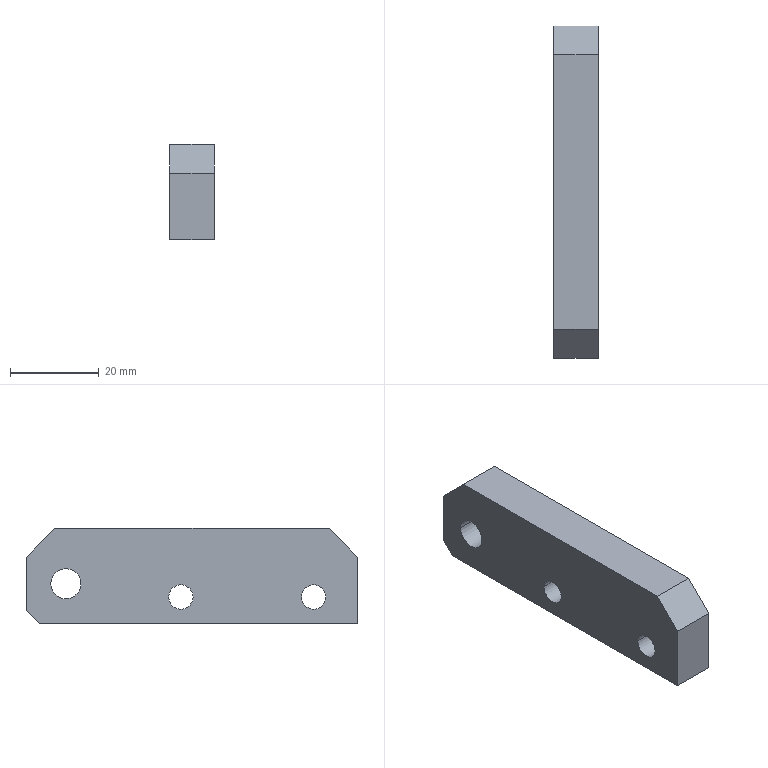Part | NX | features 001 2 | 1 solid | 15 faces | box 10 x 75 x 21.5 mm | volume 14819 mm3 | plane 9 | cylinder 6 | commonest cylinder face diameters 5.5 x4 6.8 x2
STEP:
#1=CARTESIAN_POINT('',(-195.,37.25,-6.));
#2=VERTEX_POINT('',#1);
#3=CARTESIAN_POINT('',(-205.,37.25,-6.));
#4=VERTEX_POINT('',#3);
#5=CARTESIAN_POINT('',(-195.,37.25,-6.));
#6=DIRECTION('',(-1.,0.,0.));
#7=VECTOR('',#6,1000.);
#8=LINE('',#5,#7);
#9=EDGE_CURVE('',#2,#4,#8,.T.);
#10=ORIENTED_EDGE('',*,*,#9,.F.);
#11=CARTESIAN_POINT('',(-195.,42.75,-6.));
#12=VERTEX_POINT('',#11);
#13=CARTESIAN_POINT('',(-195.,40.,-6.));
#14=DIRECTION('',(-1.,0.,0.));
#15=DIRECTION('',(0.,1.,0.));
#16=AXIS2_PLACEMENT_3D('',#13,#14,#15);
#17=CIRCLE('',#16,2.75);
#18=EDGE_CURVE('',#12,#2,#17,.T.);
#19=ORIENTED_EDGE('',*,*,#18,.F.);
#20=CARTESIAN_POINT('',(-205.,42.75,-6.));
#21=VERTEX_POINT('',#20);
#22=CARTESIAN_POINT('',(-195.,42.75,-6.));
#23=DIRECTION('',(-1.,0.,0.));
#24=VECTOR('',#23,1000.);
#25=LINE('',#22,#24);
#26=EDGE_CURVE('',#21,#12,#25,.F.);
#27=ORIENTED_EDGE('',*,*,#26,.F.);
#28=CARTESIAN_POINT('',(-205.,40.,-6.));
#29=DIRECTION('',(1.,0.,0.));
#30=DIRECTION('',(0.,-1.,0.));
#31=AXIS2_PLACEMENT_3D('',#28,#29,#30);
#32=CIRCLE('',#31,2.75);
#33=EDGE_CURVE('',#4,#21,#32,.T.);
#34=ORIENTED_EDGE('',*,*,#33,.F.);
#35=EDGE_LOOP('',(#10,#19,#27,#34));
#36=FACE_BOUND('',#35,.T.);
#37=CARTESIAN_POINT('',(-195.,40.,-6.));
#38=DIRECTION('',(1.,0.,0.));
#39=DIRECTION('',(0.,1.,0.));
#40=AXIS2_PLACEMENT_3D('',#37,#38,#39);
#41=CYLINDRICAL_SURFACE('',#40,2.75);
#42=ADVANCED_FACE('',(#36),#41,.F.);
#43=CARTESIAN_POINT('',(-205.,40.,-6.));
#44=DIRECTION('',(1.,0.,0.));
#45=DIRECTION('',(0.,1.,0.));
#46=AXIS2_PLACEMENT_3D('',#43,#44,#45);
#47=CIRCLE('',#46,2.75);
#48=EDGE_CURVE('',#21,#4,#47,.T.);
#49=ORIENTED_EDGE('',*,*,#48,.F.);
#50=ORIENTED_EDGE('',*,*,#26,.T.);
#51=CARTESIAN_POINT('',(-195.,40.,-6.));
#52=DIRECTION('',(-1.,0.,0.));
#53=DIRECTION('',(0.,-1.,0.));
#54=AXIS2_PLACEMENT_3D('',#51,#52,#53);
#55=CIRCLE('',#54,2.75);
#56=EDGE_CURVE('',#2,#12,#55,.T.);
#57=ORIENTED_EDGE('',*,*,#56,.F.);
#58=ORIENTED_EDGE('',*,*,#9,.T.);
#59=EDGE_LOOP('',(#49,#50,#57,#58));
#60=FACE_BOUND('',#59,.T.);
#61=CARTESIAN_POINT('',(-195.,40.,-6.));
#62=DIRECTION('',(1.,0.,0.));
#63=DIRECTION('',(0.,1.,0.));
#64=AXIS2_PLACEMENT_3D('',#61,#62,#63);
#65=CYLINDRICAL_SURFACE('',#64,2.75);
#66=ADVANCED_FACE('',(#60),#65,.F.);
#67=CARTESIAN_POINT('',(-205.,7.25,-6.));
#68=VERTEX_POINT('',#67);
#69=CARTESIAN_POINT('',(-195.,7.25,-6.));
#70=VERTEX_POINT('',#69);
#71=CARTESIAN_POINT('',(-195.,7.25,-6.));
#72=DIRECTION('',(-1.,0.,0.));
#73=VECTOR('',#72,1000.);
#74=LINE('',#71,#73);
#75=EDGE_CURVE('',#68,#70,#74,.F.);
#76=ORIENTED_EDGE('',*,*,#75,.T.);
#77=CARTESIAN_POINT('',(-195.,12.75,-6.));
#78=VERTEX_POINT('',#77);
#79=CARTESIAN_POINT('',(-195.,10.,-6.));
#80=DIRECTION('',(-1.,0.,0.));
#81=DIRECTION('',(0.,1.,0.));
#82=AXIS2_PLACEMENT_3D('',#79,#80,#81);
#83=CIRCLE('',#82,2.75);
#84=EDGE_CURVE('',#78,#70,#83,.T.);
#85=ORIENTED_EDGE('',*,*,#84,.F.);
#86=CARTESIAN_POINT('',(-205.,12.75,-6.));
#87=VERTEX_POINT('',#86);
#88=CARTESIAN_POINT('',(-195.,12.75,-6.));
#89=DIRECTION('',(-1.,0.,0.));
#90=VECTOR('',#89,1000.);
#91=LINE('',#88,#90);
#92=EDGE_CURVE('',#78,#87,#91,.T.);
#93=ORIENTED_EDGE('',*,*,#92,.T.);
#94=CARTESIAN_POINT('',(-205.,10.,-6.));
#95=DIRECTION('',(1.,0.,0.));
#96=DIRECTION('',(0.,-1.,0.));
#97=AXIS2_PLACEMENT_3D('',#94,#95,#96);
#98=CIRCLE('',#97,2.75);
#99=EDGE_CURVE('',#68,#87,#98,.T.);
#100=ORIENTED_EDGE('',*,*,#99,.F.);
#101=EDGE_LOOP('',(#76,#85,#93,#100));
#102=FACE_BOUND('',#101,.T.);
#103=CARTESIAN_POINT('',(-195.,10.,-6.));
#104=DIRECTION('',(1.,0.,0.));
#105=DIRECTION('',(0.,1.,0.));
#106=AXIS2_PLACEMENT_3D('',#103,#104,#105);
#107=CYLINDRICAL_SURFACE('',#106,2.75);
#108=ADVANCED_FACE('',(#102),#107,.F.);
#109=CARTESIAN_POINT('',(-205.,10.,-6.));
#110=DIRECTION('',(1.,0.,0.));
#111=DIRECTION('',(0.,1.,0.));
#112=AXIS2_PLACEMENT_3D('',#109,#110,#111);
#113=CIRCLE('',#112,2.75);
#114=EDGE_CURVE('',#87,#68,#113,.T.);
#115=ORIENTED_EDGE('',*,*,#114,.F.);
#116=ORIENTED_EDGE('',*,*,#92,.F.);
#117=CARTESIAN_POINT('',(-195.,10.,-6.));
#118=DIRECTION('',(-1.,0.,0.));
#119=DIRECTION('',(0.,-1.,0.));
#120=AXIS2_PLACEMENT_3D('',#117,#118,#119);
#121=CIRCLE('',#120,2.75);
#122=EDGE_CURVE('',#70,#78,#121,.T.);
#123=ORIENTED_EDGE('',*,*,#122,.F.);
#124=ORIENTED_EDGE('',*,*,#75,.F.);
#125=EDGE_LOOP('',(#115,#116,#123,#124));
#126=FACE_BOUND('',#125,.T.);
#127=CARTESIAN_POINT('',(-195.,10.,-6.));
#128=DIRECTION('',(1.,0.,0.));
#129=DIRECTION('',(0.,1.,0.));
#130=AXIS2_PLACEMENT_3D('',#127,#128,#129);
#131=CYLINDRICAL_SURFACE('',#130,2.75);
#132=ADVANCED_FACE('',(#126),#131,.F.);
#133=CARTESIAN_POINT('',(-205.,69.4,-3.));
#134=VERTEX_POINT('',#133);
#135=CARTESIAN_POINT('',(-205.,62.6,-3.));
#136=VERTEX_POINT('',#135);
#137=CARTESIAN_POINT('',(-205.,66.,-3.));
#138=DIRECTION('',(1.,0.,0.));
#139=DIRECTION('',(0.,1.,0.));
#140=AXIS2_PLACEMENT_3D('',#137,#138,#139);
#141=CIRCLE('',#140,3.4);
#142=EDGE_CURVE('',#134,#136,#141,.T.);
#143=ORIENTED_EDGE('',*,*,#142,.F.);
#144=CARTESIAN_POINT('',(-195.,69.4,-3.));
#145=VERTEX_POINT('',#144);
#146=CARTESIAN_POINT('',(-195.,69.4,-3.));
#147=DIRECTION('',(-1.,0.,0.));
#148=VECTOR('',#147,1000.);
#149=LINE('',#146,#148);
#150=EDGE_CURVE('',#134,#145,#149,.F.);
#151=ORIENTED_EDGE('',*,*,#150,.T.);
#152=CARTESIAN_POINT('',(-195.,62.6,-3.));
#153=VERTEX_POINT('',#152);
#154=CARTESIAN_POINT('',(-195.,66.,-3.));
#155=DIRECTION('',(-1.,0.,0.));
#156=DIRECTION('',(0.,-1.,0.));
#157=AXIS2_PLACEMENT_3D('',#154,#155,#156);
#158=CIRCLE('',#157,3.4);
#159=EDGE_CURVE('',#153,#145,#158,.T.);
#160=ORIENTED_EDGE('',*,*,#159,.F.);
#161=CARTESIAN_POINT('',(-195.,62.6,-3.));
#162=DIRECTION('',(-1.,0.,0.));
#163=VECTOR('',#162,1000.);
#164=LINE('',#161,#163);
#165=EDGE_CURVE('',#153,#136,#164,.T.);
#166=ORIENTED_EDGE('',*,*,#165,.T.);
#167=EDGE_LOOP('',(#143,#151,#160,#166));
#168=FACE_BOUND('',#167,.T.);
#169=CARTESIAN_POINT('',(-195.,66.,-3.));
#170=DIRECTION('',(1.,0.,0.));
#171=DIRECTION('',(0.,1.,0.));
#172=AXIS2_PLACEMENT_3D('',#169,#170,#171);
#173=CYLINDRICAL_SURFACE('',#172,3.4);
#174=ADVANCED_FACE('',(#168),#173,.F.);
#175=CARTESIAN_POINT('',(-195.,6.5,9.5));
#176=VERTEX_POINT('',#175);
#177=CARTESIAN_POINT('',(-205.,6.5,9.5));
#178=VERTEX_POINT('',#177);
#179=CARTESIAN_POINT('',(-195.,6.5,9.5));
#180=DIRECTION('',(1.,0.,0.));
#181=VECTOR('',#180,1000.);
#182=LINE('',#179,#181);
#183=EDGE_CURVE('',#176,#178,#182,.F.);
#184=ORIENTED_EDGE('',*,*,#183,.T.);
#185=CARTESIAN_POINT('',(-205.,0.,3.));
#186=VERTEX_POINT('',#185);
#187=CARTESIAN_POINT('',(-205.,0.,3.));
#188=DIRECTION('',(0.,0.7071,0.7071));
#189=VECTOR('',#188,1000.);
#190=LINE('',#187,#189);
#191=EDGE_CURVE('',#186,#178,#190,.T.);
#192=ORIENTED_EDGE('',*,*,#191,.F.);
#193=CARTESIAN_POINT('',(-195.,0.,3.));
#194=VERTEX_POINT('',#193);
#195=CARTESIAN_POINT('',(-205.,0.,3.));
#196=DIRECTION('',(1.,0.,0.));
#197=VECTOR('',#196,1000.);
#198=LINE('',#195,#197);
#199=EDGE_CURVE('',#186,#194,#198,.T.);
#200=ORIENTED_EDGE('',*,*,#199,.T.);
#201=CARTESIAN_POINT('',(-195.,3.,6.));
#202=DIRECTION('',(0.,-0.7071,-0.7071));
#203=VECTOR('',#202,1000.);
#204=LINE('',#201,#203);
#205=EDGE_CURVE('',#176,#194,#204,.T.);
#206=ORIENTED_EDGE('',*,*,#205,.F.);
#207=EDGE_LOOP('',(#184,#192,#200,#206));
#208=FACE_BOUND('',#207,.T.);
#209=CARTESIAN_POINT('',(-195.,0.,3.));
#210=DIRECTION('',(0.,0.7071,-0.7071));
#211=DIRECTION('',(-1.,0.,0.));
#212=AXIS2_PLACEMENT_3D('',#209,#210,#211);
#213=PLANE('',#212);
#214=ADVANCED_FACE('',(#208),#213,.F.);
#215=CARTESIAN_POINT('',(-195.,72.,-12.));
#216=VERTEX_POINT('',#215);
#217=CARTESIAN_POINT('',(-205.,72.,-12.));
#218=VERTEX_POINT('',#217);
#219=CARTESIAN_POINT('',(-195.,72.,-12.));
#220=DIRECTION('',(-1.,0.,0.));
#221=VECTOR('',#220,1000.);
#222=LINE('',#219,#221);
#223=EDGE_CURVE('',#216,#218,#222,.T.);
#224=ORIENTED_EDGE('',*,*,#223,.F.);
#225=CARTESIAN_POINT('',(-195.,0.,-12.));
#226=VERTEX_POINT('',#225);
#227=CARTESIAN_POINT('',(-195.,72.,-12.));
#228=DIRECTION('',(0.,-1.,0.));
#229=VECTOR('',#228,1000.);
#230=LINE('',#227,#229);
#231=EDGE_CURVE('',#216,#226,#230,.T.);
#232=ORIENTED_EDGE('',*,*,#231,.T.);
#233=CARTESIAN_POINT('',(-205.,0.,-12.));
#234=VERTEX_POINT('',#233);
#235=CARTESIAN_POINT('',(-205.,0.,-12.));
#236=DIRECTION('',(1.,0.,0.));
#237=VECTOR('',#236,1000.);
#238=LINE('',#235,#237);
#239=EDGE_CURVE('',#234,#226,#238,.T.);
#240=ORIENTED_EDGE('',*,*,#239,.F.);
#241=CARTESIAN_POINT('',(-205.,72.,-12.));
#242=DIRECTION('',(0.,-1.,0.));
#243=VECTOR('',#242,1000.);
#244=LINE('',#241,#243);
#245=EDGE_CURVE('',#218,#234,#244,.T.);
#246=ORIENTED_EDGE('',*,*,#245,.F.);
#247=EDGE_LOOP('',(#224,#232,#240,#246));
#248=FACE_BOUND('',#247,.T.);
#249=CARTESIAN_POINT('',(-195.,75.,-12.));
#250=DIRECTION('',(0.,0.,1.));
#251=DIRECTION('',(0.,-1.,0.));
#252=AXIS2_PLACEMENT_3D('',#249,#250,#251);
#253=PLANE('',#252);
#254=ADVANCED_FACE('',(#248),#253,.F.);
#255=ORIENTED_EDGE('',*,*,#223,.T.);
#256=CARTESIAN_POINT('',(-205.,75.,-9.));
#257=VERTEX_POINT('',#256);
#258=CARTESIAN_POINT('',(-205.,75.,-9.));
#259=DIRECTION('',(0.,-0.7071,-0.7071));
#260=VECTOR('',#259,1000.);
#261=LINE('',#258,#260);
#262=EDGE_CURVE('',#257,#218,#261,.T.);
#263=ORIENTED_EDGE('',*,*,#262,.F.);
#264=CARTESIAN_POINT('',(-195.,75.,-9.));
#265=VERTEX_POINT('',#264);
#266=CARTESIAN_POINT('',(-205.,75.,-9.));
#267=DIRECTION('',(1.,0.,0.));
#268=VECTOR('',#267,1000.);
#269=LINE('',#266,#268);
#270=EDGE_CURVE('',#257,#265,#269,.T.);
#271=ORIENTED_EDGE('',*,*,#270,.T.);
#272=CARTESIAN_POINT('',(-195.,72.,-12.));
#273=DIRECTION('',(0.,0.7071,0.7071));
#274=VECTOR('',#273,1000.);
#275=LINE('',#272,#274);
#276=EDGE_CURVE('',#216,#265,#275,.T.);
#277=ORIENTED_EDGE('',*,*,#276,.F.);
#278=EDGE_LOOP('',(#255,#263,#271,#277));
#279=FACE_BOUND('',#278,.T.);
#280=CARTESIAN_POINT('',(-195.,75.,-9.));
#281=DIRECTION('',(0.,-0.7071,0.7071));
#282=DIRECTION('',(-1.,0.,0.));
#283=AXIS2_PLACEMENT_3D('',#280,#281,#282);
#284=PLANE('',#283);
#285=ADVANCED_FACE('',(#279),#284,.F.);
#286=ORIENTED_EDGE('',*,*,#270,.F.);
#287=CARTESIAN_POINT('',(-205.,75.,3.));
#288=VERTEX_POINT('',#287);
#289=CARTESIAN_POINT('',(-205.,75.,3.));
#290=DIRECTION('',(0.,0.,-1.));
#291=VECTOR('',#290,1000.);
#292=LINE('',#289,#291);
#293=EDGE_CURVE('',#288,#257,#292,.T.);
#294=ORIENTED_EDGE('',*,*,#293,.F.);
#295=CARTESIAN_POINT('',(-195.,75.,3.));
#296=VERTEX_POINT('',#295);
#297=CARTESIAN_POINT('',(-195.,75.,3.));
#298=DIRECTION('',(-1.,0.,0.));
#299=VECTOR('',#298,1000.);
#300=LINE('',#297,#299);
#301=EDGE_CURVE('',#296,#288,#300,.T.);
#302=ORIENTED_EDGE('',*,*,#301,.F.);
#303=CARTESIAN_POINT('',(-195.,75.,3.));
#304=DIRECTION('',(0.,0.,-1.));
#305=VECTOR('',#304,1000.);
#306=LINE('',#303,#305);
#307=EDGE_CURVE('',#296,#265,#306,.T.);
#308=ORIENTED_EDGE('',*,*,#307,.T.);
#309=EDGE_LOOP('',(#286,#294,#302,#308));
#310=FACE_BOUND('',#309,.T.);
#311=CARTESIAN_POINT('',(-195.,75.,-12.));
#312=DIRECTION('',(0.,-1.,0.));
#313=DIRECTION('',(1.,0.,0.));
#314=AXIS2_PLACEMENT_3D('',#311,#312,#313);
#315=PLANE('',#314);
#316=ADVANCED_FACE('',(#310),#315,.F.);
#317=ORIENTED_EDGE('',*,*,#301,.T.);
#318=CARTESIAN_POINT('',(-205.,68.5,9.5));
#319=VERTEX_POINT('',#318);
#320=CARTESIAN_POINT('',(-205.,72.,6.));
#321=DIRECTION('',(0.,0.7071,-0.7071));
#322=VECTOR('',#321,1000.);
#323=LINE('',#320,#322);
#324=EDGE_CURVE('',#319,#288,#323,.T.);
#325=ORIENTED_EDGE('',*,*,#324,.F.);
#326=CARTESIAN_POINT('',(-195.,68.5,9.5));
#327=VERTEX_POINT('',#326);
#328=CARTESIAN_POINT('',(-195.,68.5,9.5));
#329=DIRECTION('',(-1.,0.,0.));
#330=VECTOR('',#329,1000.);
#331=LINE('',#328,#330);
#332=EDGE_CURVE('',#319,#327,#331,.F.);
#333=ORIENTED_EDGE('',*,*,#332,.T.);
#334=CARTESIAN_POINT('',(-195.,75.,3.));
#335=DIRECTION('',(0.,-0.7071,0.7071));
#336=VECTOR('',#335,1000.);
#337=LINE('',#334,#336);
#338=EDGE_CURVE('',#296,#327,#337,.T.);
#339=ORIENTED_EDGE('',*,*,#338,.F.);
#340=EDGE_LOOP('',(#317,#325,#333,#339));
#341=FACE_BOUND('',#340,.T.);
#342=CARTESIAN_POINT('',(-195.,72.,6.));
#343=DIRECTION('',(0.,-0.7071,-0.7071));
#344=DIRECTION('',(-1.,0.,0.));
#345=AXIS2_PLACEMENT_3D('',#342,#343,#344);
#346=PLANE('',#345);
#347=ADVANCED_FACE('',(#341),#346,.F.);
#348=ORIENTED_EDGE('',*,*,#183,.F.);
#349=CARTESIAN_POINT('',(-195.,37.5,9.5));
#350=DIRECTION('',(0.,-1.,0.));
#351=VECTOR('',#350,1000.);
#352=LINE('',#349,#351);
#353=EDGE_CURVE('',#176,#327,#352,.F.);
#354=ORIENTED_EDGE('',*,*,#353,.T.);
#355=ORIENTED_EDGE('',*,*,#332,.F.);
#356=CARTESIAN_POINT('',(-205.,37.5,9.5));
#357=DIRECTION('',(0.,-1.,0.));
#358=VECTOR('',#357,1000.);
#359=LINE('',#356,#358);
#360=EDGE_CURVE('',#178,#319,#359,.F.);
#361=ORIENTED_EDGE('',*,*,#360,.F.);
#362=EDGE_LOOP('',(#348,#354,#355,#361));
#363=FACE_BOUND('',#362,.T.);
#364=CARTESIAN_POINT('',(-200.,25.,9.5));
#365=DIRECTION('',(0.,0.,1.));
#366=DIRECTION('',(0.5212,0.8534,0.));
#367=AXIS2_PLACEMENT_3D('',#364,#365,#366);
#368=PLANE('',#367);
#369=ADVANCED_FACE('',(#363),#368,.T.);
#370=ORIENTED_EDGE('',*,*,#18,.T.);
#371=ORIENTED_EDGE('',*,*,#56,.T.);
#372=EDGE_LOOP('',(#370,#371));
#373=FACE_BOUND('',#372,.T.);
#374=ORIENTED_EDGE('',*,*,#84,.T.);
#375=ORIENTED_EDGE('',*,*,#122,.T.);
#376=EDGE_LOOP('',(#374,#375));
#377=FACE_BOUND('',#376,.T.);
#378=CARTESIAN_POINT('',(-195.,66.,-3.));
#379=DIRECTION('',(-1.,0.,0.));
#380=DIRECTION('',(0.,1.,0.));
#381=AXIS2_PLACEMENT_3D('',#378,#379,#380);
#382=CIRCLE('',#381,3.4);
#383=EDGE_CURVE('',#145,#153,#382,.T.);
#384=ORIENTED_EDGE('',*,*,#383,.T.);
#385=ORIENTED_EDGE('',*,*,#159,.T.);
#386=EDGE_LOOP('',(#384,#385));
#387=FACE_BOUND('',#386,.T.);
#388=ORIENTED_EDGE('',*,*,#205,.T.);
#389=CARTESIAN_POINT('',(-195.,0.,-12.));
#390=DIRECTION('',(0.,0.,1.));
#391=VECTOR('',#390,1000.);
#392=LINE('',#389,#391);
#393=EDGE_CURVE('',#226,#194,#392,.T.);
#394=ORIENTED_EDGE('',*,*,#393,.F.);
#395=ORIENTED_EDGE('',*,*,#231,.F.);
#396=ORIENTED_EDGE('',*,*,#276,.T.);
#397=ORIENTED_EDGE('',*,*,#307,.F.);
#398=ORIENTED_EDGE('',*,*,#338,.T.);
#399=ORIENTED_EDGE('',*,*,#353,.F.);
#400=EDGE_LOOP('',(#388,#394,#395,#396,#397,#398,#399));
#401=FACE_BOUND('',#400,.T.);
#402=CARTESIAN_POINT('',(-195.,37.5,-3.));
#403=DIRECTION('',(1.,0.,0.));
#404=DIRECTION('',(0.,1.,0.));
#405=AXIS2_PLACEMENT_3D('',#402,#403,#404);
#406=PLANE('',#405);
#407=ADVANCED_FACE('',(#373,#377,#387,#401),#406,.T.);
#408=ORIENTED_EDGE('',*,*,#199,.F.);
#409=CARTESIAN_POINT('',(-205.,0.,-12.));
#410=DIRECTION('',(0.,0.,1.));
#411=VECTOR('',#410,1000.);
#412=LINE('',#409,#411);
#413=EDGE_CURVE('',#234,#186,#412,.T.);
#414=ORIENTED_EDGE('',*,*,#413,.F.);
#415=ORIENTED_EDGE('',*,*,#239,.T.);
#416=ORIENTED_EDGE('',*,*,#393,.T.);
#417=EDGE_LOOP('',(#408,#414,#415,#416));
#418=FACE_BOUND('',#417,.T.);
#419=CARTESIAN_POINT('',(-195.,0.,-12.));
#420=DIRECTION('',(0.,1.,0.));
#421=DIRECTION('',(-1.,0.,0.));
#422=AXIS2_PLACEMENT_3D('',#419,#420,#421);
#423=PLANE('',#422);
#424=ADVANCED_FACE('',(#418),#423,.F.);
#425=ORIENTED_EDGE('',*,*,#33,.T.);
#426=ORIENTED_EDGE('',*,*,#48,.T.);
#427=EDGE_LOOP('',(#425,#426));
#428=FACE_BOUND('',#427,.T.);
#429=ORIENTED_EDGE('',*,*,#99,.T.);
#430=ORIENTED_EDGE('',*,*,#114,.T.);
#431=EDGE_LOOP('',(#429,#430));
#432=FACE_BOUND('',#431,.T.);
#433=CARTESIAN_POINT('',(-205.,66.,-3.));
#434=DIRECTION('',(1.,0.,0.));
#435=DIRECTION('',(0.,-1.,0.));
#436=AXIS2_PLACEMENT_3D('',#433,#434,#435);
#437=CIRCLE('',#436,3.4);
#438=EDGE_CURVE('',#136,#134,#437,.T.);
#439=ORIENTED_EDGE('',*,*,#438,.T.);
#440=ORIENTED_EDGE('',*,*,#142,.T.);
#441=EDGE_LOOP('',(#439,#440));
#442=FACE_BOUND('',#441,.T.);
#443=ORIENTED_EDGE('',*,*,#191,.T.);
#444=ORIENTED_EDGE('',*,*,#360,.T.);
#445=ORIENTED_EDGE('',*,*,#324,.T.);
#446=ORIENTED_EDGE('',*,*,#293,.T.);
#447=ORIENTED_EDGE('',*,*,#262,.T.);
#448=ORIENTED_EDGE('',*,*,#245,.T.);
#449=ORIENTED_EDGE('',*,*,#413,.T.);
#450=EDGE_LOOP('',(#443,#444,#445,#446,#447,#448,#449));
#451=FACE_BOUND('',#450,.T.);
#452=CARTESIAN_POINT('',(-205.,37.5,-3.));
#453=DIRECTION('',(1.,0.,0.));
#454=DIRECTION('',(0.,1.,0.));
#455=AXIS2_PLACEMENT_3D('',#452,#453,#454);
#456=PLANE('',#455);
#457=ADVANCED_FACE('',(#428,#432,#442,#451),#456,.F.);
#458=ORIENTED_EDGE('',*,*,#165,.F.);
#459=ORIENTED_EDGE('',*,*,#383,.F.);
#460=ORIENTED_EDGE('',*,*,#150,.F.);
#461=ORIENTED_EDGE('',*,*,#438,.F.);
#462=EDGE_LOOP('',(#458,#459,#460,#461));
#463=FACE_BOUND('',#462,.T.);
#464=CARTESIAN_POINT('',(-195.,66.,-3.));
#465=DIRECTION('',(1.,0.,0.));
#466=DIRECTION('',(0.,1.,0.));
#467=AXIS2_PLACEMENT_3D('',#464,#465,#466);
#468=CYLINDRICAL_SURFACE('',#467,3.4);
#469=ADVANCED_FACE('',(#463),#468,.F.);
#470=CLOSED_SHELL('',(#42,#66,#108,#132,#174,#214,#254,#285,#316,#347,#369,#407,#424,#457,#469));
#471=MANIFOLD_SOLID_BREP('',#470);
#472=(LENGTH_UNIT()NAMED_UNIT(*)SI_UNIT(.MILLI.,.METRE.));
#473=UNCERTAINTY_MEASURE_WITH_UNIT(LENGTH_MEASURE(0.00001),#472,'','');
#474=(NAMED_UNIT(*)PLANE_ANGLE_UNIT()SI_UNIT($,.RADIAN.));
#475=(NAMED_UNIT(*)SI_UNIT($,.STERADIAN.)SOLID_ANGLE_UNIT());
#476=(GEOMETRIC_REPRESENTATION_CONTEXT(3)GLOBAL_UNCERTAINTY_ASSIGNED_CONTEXT((#473))GLOBAL_UNIT_ASSIGNED_CONTEXT((#472,#474,#475))REPRESENTATION_CONTEXT('',''));
#477=ADVANCED_BREP_SHAPE_REPRESENTATION('',(#471),#476);